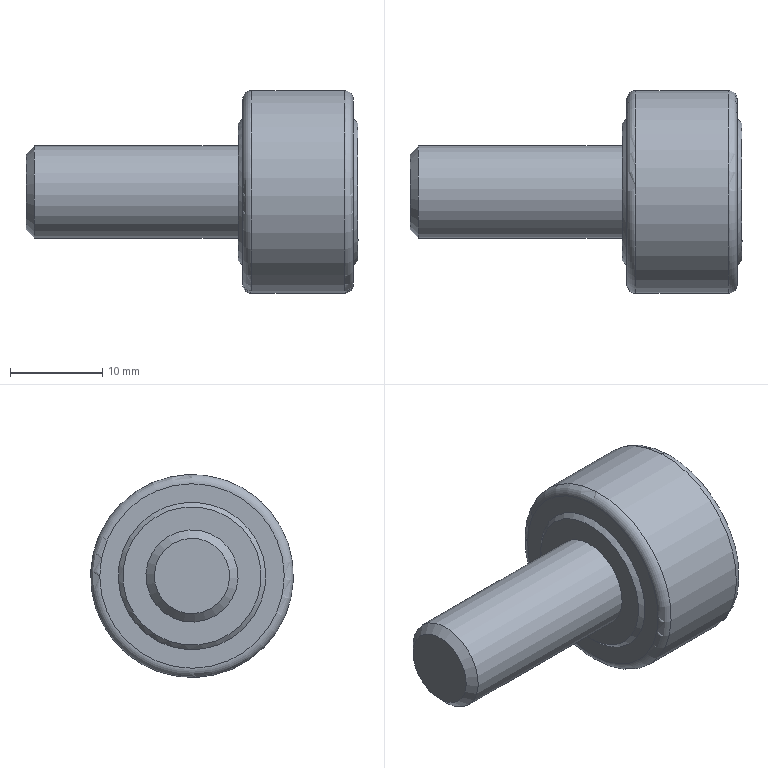Part | NX | features CFFRC10-22 2 | 1 solid | 24 faces | box 36 x 22 x 22 mm | volume 6364 mm3 | plane 14 | cone 4 | cylinder 4 | torus 2 | commonest cylinder face diameters 2 x1 4 x1 10 x1 22 x1
STEP:
#1=CARTESIAN_POINT('',(-25.5,-117.523,-671.264));
#2=VERTEX_POINT('',#1);
#3=CARTESIAN_POINT('',(-25.5,-120.421,-674.136));
#4=DIRECTION('',(-1.,0.,0.));
#5=DIRECTION('',(0.,0.7102,0.704));
#6=AXIS2_PLACEMENT_3D('',#3,#4,#5);
#7=CIRCLE('',#6,4.08);
#8=EDGE_CURVE('',#2,#2,#7,.T.);
#9=ORIENTED_EDGE('',*,*,#8,.T.);
#10=EDGE_LOOP('',(#9));
#11=FACE_BOUND('',#10,.T.);
#12=CARTESIAN_POINT('',(-25.5,-121.857,-672.688));
#13=DIRECTION('',(-1.,0.,0.));
#14=DIRECTION('',(0.,-0.7102,-0.704));
#15=AXIS2_PLACEMENT_3D('',#12,#13,#14);
#16=PLANE('',#15);
#17=ADVANCED_FACE('',(#11),#16,.T.);
#18=CARTESIAN_POINT('',(-24.58,-123.972,-677.656));
#19=VERTEX_POINT('',#18);
#20=CARTESIAN_POINT('',(-24.58,-120.421,-674.136));
#21=DIRECTION('',(-1.,0.,0.));
#22=DIRECTION('',(0.,-0.7102,-0.704));
#23=AXIS2_PLACEMENT_3D('',#20,#21,#22);
#24=CIRCLE('',#23,5.);
#25=EDGE_CURVE('',#19,#19,#24,.T.);
#26=ORIENTED_EDGE('',*,*,#25,.T.);
#27=EDGE_LOOP('',(#26));
#28=FACE_BOUND('',#27,.T.);
#29=ORIENTED_EDGE('',*,*,#8,.F.);
#30=EDGE_LOOP('',(#29));
#31=FACE_BOUND('',#30,.T.);
#32=CARTESIAN_POINT('',(-25.54,-120.421,-674.136));
#33=DIRECTION('',(1.,0.,0.));
#34=DIRECTION('',(0.,0.7102,0.704));
#35=AXIS2_PLACEMENT_3D('',#32,#33,#34);
#36=CONICAL_SURFACE('',#35,4.04,0.7854);
#37=ADVANCED_FACE('',(#28,#31),#36,.T.);
#38=ORIENTED_EDGE('',*,*,#25,.F.);
#39=EDGE_LOOP('',(#38));
#40=FACE_BOUND('',#39,.T.);
#41=CARTESIAN_POINT('',(-2.5,-116.87,-670.616));
#42=VERTEX_POINT('',#41);
#43=CARTESIAN_POINT('',(-2.5,-120.421,-674.136));
#44=DIRECTION('',(1.,0.,0.));
#45=DIRECTION('',(0.,0.7102,0.704));
#46=AXIS2_PLACEMENT_3D('',#43,#44,#45);
#47=CIRCLE('',#46,5.);
#48=EDGE_CURVE('',#42,#42,#47,.T.);
#49=ORIENTED_EDGE('',*,*,#48,.F.);
#50=EDGE_LOOP('',(#49));
#51=FACE_BOUND('',#50,.T.);
#52=CARTESIAN_POINT('',(-13.54,-120.421,-674.136));
#53=DIRECTION('',(-1.,0.,0.));
#54=DIRECTION('',(0.,-0.7102,-0.704));
#55=AXIS2_PLACEMENT_3D('',#52,#53,#54);
#56=CYLINDRICAL_SURFACE('',#55,5.);
#57=ADVANCED_FACE('',(#40,#51),#56,.T.);
#58=ORIENTED_EDGE('',*,*,#48,.T.);
#59=EDGE_LOOP('',(#58));
#60=FACE_BOUND('',#59,.T.);
#61=CARTESIAN_POINT('',(-2.5,-115.094,-668.856));
#62=VERTEX_POINT('',#61);
#63=CARTESIAN_POINT('',(-2.5,-120.421,-674.136));
#64=DIRECTION('',(-1.,0.,0.));
#65=DIRECTION('',(0.,0.7102,0.704));
#66=AXIS2_PLACEMENT_3D('',#63,#64,#65);
#67=CIRCLE('',#66,7.5);
#68=EDGE_CURVE('',#62,#62,#67,.T.);
#69=ORIENTED_EDGE('',*,*,#68,.T.);
#70=EDGE_LOOP('',(#69));
#71=FACE_BOUND('',#70,.T.);
#72=CARTESIAN_POINT('',(-2.5,-124.821,-669.698));
#73=DIRECTION('',(-1.,0.,0.));
#74=DIRECTION('',(0.,-0.7102,-0.704));
#75=AXIS2_PLACEMENT_3D('',#72,#73,#74);
#76=PLANE('',#75);
#77=ADVANCED_FACE('',(#60,#71),#76,.T.);
#78=ORIENTED_EDGE('',*,*,#68,.F.);
#79=EDGE_LOOP('',(#78));
#80=FACE_BOUND('',#79,.T.);
#81=CARTESIAN_POINT('',(-2.,-126.102,-679.768));
#82=VERTEX_POINT('',#81);
#83=CARTESIAN_POINT('',(-2.,-120.421,-674.136));
#84=DIRECTION('',(1.,0.,0.));
#85=DIRECTION('',(0.,-0.7102,-0.704));
#86=AXIS2_PLACEMENT_3D('',#83,#84,#85);
#87=CIRCLE('',#86,8.);
#88=EDGE_CURVE('',#82,#82,#87,.T.);
#89=ORIENTED_EDGE('',*,*,#88,.F.);
#90=EDGE_LOOP('',(#89));
#91=FACE_BOUND('',#90,.T.);
#92=CARTESIAN_POINT('',(-2.54,-120.421,-674.136));
#93=DIRECTION('',(1.,0.,0.));
#94=DIRECTION('',(0.,0.7102,0.704));
#95=AXIS2_PLACEMENT_3D('',#92,#93,#94);
#96=CONICAL_SURFACE('',#95,7.46,0.7854);
#97=ADVANCED_FACE('',(#80,#91),#96,.T.);
#98=ORIENTED_EDGE('',*,*,#88,.T.);
#99=EDGE_LOOP('',(#98));
#100=FACE_BOUND('',#99,.T.);
#101=CARTESIAN_POINT('',(-2.,-113.319,-667.096));
#102=VERTEX_POINT('',#101);
#103=CARTESIAN_POINT('',(-2.,-120.421,-674.136));
#104=DIRECTION('',(-1.,0.,0.));
#105=DIRECTION('',(0.,0.7102,0.704));
#106=AXIS2_PLACEMENT_3D('',#103,#104,#105);
#107=CIRCLE('',#106,10.);
#108=EDGE_CURVE('',#102,#102,#107,.T.);
#109=ORIENTED_EDGE('',*,*,#108,.T.);
#110=EDGE_LOOP('',(#109));
#111=FACE_BOUND('',#110,.T.);
#112=CARTESIAN_POINT('',(-2.,-126.757,-667.745));
#113=DIRECTION('',(-1.,0.,0.));
#114=DIRECTION('',(0.,-0.704,0.7102));
#115=AXIS2_PLACEMENT_3D('',#112,#113,#114);
#116=PLANE('',#115);
#117=ADVANCED_FACE('',(#100,#111),#116,.T.);
#118=CARTESIAN_POINT('',(4.,-123.935,-669.171));
#119=VERTEX_POINT('',#118);
#120=CARTESIAN_POINT('',(4.,-124.645,-669.875));
#121=DIRECTION('',(0.,0.704,-0.7102));
#122=DIRECTION('',(0.,0.7102,0.704));
#123=AXIS2_PLACEMENT_3D('',#120,#121,#122);
#124=CIRCLE('',#123,1.);
#125=EDGE_CURVE('',#119,#119,#124,.T.);
#126=ORIENTED_EDGE('',*,*,#125,.T.);
#127=EDGE_LOOP('',(#126));
#128=FACE_BOUND('',#127,.T.);
#129=CARTESIAN_POINT('',(4.5,-124.645,-669.875));
#130=DIRECTION('',(0.,-0.704,0.7102));
#131=DIRECTION('',(0.,0.7102,0.704));
#132=AXIS2_PLACEMENT_3D('',#129,#130,#131);
#133=PLANE('',#132);
#134=ADVANCED_FACE('',(#128),#133,.F.);
#135=CARTESIAN_POINT('',(4.,-120.93,-672.202));
#136=VERTEX_POINT('',#135);
#137=CARTESIAN_POINT('',(4.,-122.35,-673.61));
#138=VERTEX_POINT('',#137);
#139=CARTESIAN_POINT('',(4.,-120.93,-672.202));
#140=CARTESIAN_POINT('',(3.465,-120.928,-672.204));
#141=CARTESIAN_POINT('',(2.535,-122.019,-672.524));
#142=CARTESIAN_POINT('',(3.465,-122.349,-673.612));
#143=CARTESIAN_POINT('',(4.,-122.35,-673.61));
#144=B_SPLINE_CURVE_WITH_KNOTS('',3,(#139,#140,#141,#142,#143),.UNSPECIFIED.,.F.,.F.,(4,1,4),(0.,0.5,1.),.UNSPECIFIED.);
#145=EDGE_CURVE('',#136,#138,#144,.T.);
#146=ORIENTED_EDGE('',*,*,#145,.F.);
#147=CARTESIAN_POINT('',(4.,-122.35,-673.61));
#148=CARTESIAN_POINT('',(4.535,-122.349,-673.612));
#149=CARTESIAN_POINT('',(5.465,-122.019,-672.524));
#150=CARTESIAN_POINT('',(4.535,-120.928,-672.204));
#151=CARTESIAN_POINT('',(4.,-120.93,-672.202));
#152=B_SPLINE_CURVE_WITH_KNOTS('',3,(#147,#148,#149,#150,#151),.UNSPECIFIED.,.F.,.F.,(4,1,4),(0.,0.5,1.),.UNSPECIFIED.);
#153=EDGE_CURVE('',#138,#136,#152,.T.);
#154=ORIENTED_EDGE('',*,*,#153,.F.);
#155=EDGE_LOOP('',(#146,#154));
#156=FACE_BOUND('',#155,.T.);
#157=ORIENTED_EDGE('',*,*,#125,.F.);
#158=EDGE_LOOP('',(#157));
#159=FACE_BOUND('',#158,.T.);
#160=CARTESIAN_POINT('',(4.,-122.885,-671.651));
#161=DIRECTION('',(0.,-0.704,0.7102));
#162=DIRECTION('',(0.,0.7102,0.704));
#163=AXIS2_PLACEMENT_3D('',#160,#161,#162);
#164=CYLINDRICAL_SURFACE('',#163,1.);
#165=ADVANCED_FACE('',(#156,#159),#164,.F.);
#166=CARTESIAN_POINT('',(2.555,-119.,-672.728));
#167=VERTEX_POINT('',#166);
#168=CARTESIAN_POINT('',(2.555,-120.421,-674.136));
#169=DIRECTION('',(1.,0.,0.));
#170=DIRECTION('',(0.,0.7102,0.704));
#171=AXIS2_PLACEMENT_3D('',#168,#169,#170);
#172=CIRCLE('',#171,2.);
#173=EDGE_CURVE('',#167,#167,#172,.T.);
#174=ORIENTED_EDGE('',*,*,#173,.T.);
#175=EDGE_LOOP('',(#174));
#176=FACE_BOUND('',#175,.T.);
#177=CARTESIAN_POINT('',(1.4,-120.421,-674.136));
#178=VERTEX_POINT('',#177);
#179=VERTEX_LOOP('',#178);
#180=FACE_BOUND('',#179,.T.);
#181=CARTESIAN_POINT('',(1.4,-120.421,-674.136));
#182=DIRECTION('',(1.,0.,0.));
#183=DIRECTION('',(0.,0.7102,0.704));
#184=AXIS2_PLACEMENT_3D('',#181,#182,#183);
#185=CONICAL_SURFACE('',#184,0.,1.047);
#186=ADVANCED_FACE('',(#176,#180),#185,.F.);
#187=CARTESIAN_POINT('',(10.5,-117.16,-669.613));
#188=VERTEX_POINT('',#187);
#189=CARTESIAN_POINT('',(7.9,-117.16,-669.613));
#190=VERTEX_POINT('',#189);
#191=CARTESIAN_POINT('',(10.5,-117.16,-669.613));
#192=DIRECTION('',(-1.,0.,0.));
#193=VECTOR('',#192,1000.);
#194=LINE('',#191,#193);
#195=EDGE_CURVE('',#188,#190,#194,.T.);
#196=ORIENTED_EDGE('',*,*,#195,.F.);
#197=CARTESIAN_POINT('',(10.5,-119.804,-672.234));
#198=VERTEX_POINT('',#197);
#199=CARTESIAN_POINT('',(10.5,-117.16,-669.613));
#200=DIRECTION('',(0.,-0.7102,-0.704));
#201=VECTOR('',#200,1000.);
#202=LINE('',#199,#201);
#203=EDGE_CURVE('',#188,#198,#202,.T.);
#204=ORIENTED_EDGE('',*,*,#203,.T.);
#205=CARTESIAN_POINT('',(7.9,-119.804,-672.234));
#206=VERTEX_POINT('',#205);
#207=CARTESIAN_POINT('',(7.9,-119.804,-672.234));
#208=DIRECTION('',(1.,0.,0.));
#209=VECTOR('',#208,1000.);
#210=LINE('',#207,#209);
#211=EDGE_CURVE('',#206,#198,#210,.T.);
#212=ORIENTED_EDGE('',*,*,#211,.F.);
#213=CARTESIAN_POINT('',(7.9,-119.804,-672.234));
#214=DIRECTION('',(0.,0.7102,0.704));
#215=VECTOR('',#214,1000.);
#216=LINE('',#213,#215);
#217=EDGE_CURVE('',#206,#190,#216,.T.);
#218=ORIENTED_EDGE('',*,*,#217,.T.);
#219=EDGE_LOOP('',(#196,#204,#212,#218));
#220=FACE_BOUND('',#219,.T.);
#221=CARTESIAN_POINT('',(10.5,-117.16,-669.613));
#222=DIRECTION('',(0.,-0.704,0.7102));
#223=DIRECTION('',(0.,0.7102,0.704));
#224=AXIS2_PLACEMENT_3D('',#221,#222,#223);
#225=PLANE('',#224);
#226=ADVANCED_FACE('',(#220),#225,.F.);
#227=CARTESIAN_POINT('',(10.5,-115.869,-670.915));
#228=VERTEX_POINT('',#227);
#229=CARTESIAN_POINT('',(7.9,-115.869,-670.915));
#230=VERTEX_POINT('',#229);
#231=CARTESIAN_POINT('',(10.5,-115.869,-670.915));
#232=DIRECTION('',(-1.,0.,0.));
#233=VECTOR('',#232,1000.);
#234=LINE('',#231,#233);
#235=EDGE_CURVE('',#228,#230,#234,.T.);
#236=ORIENTED_EDGE('',*,*,#235,.T.);
#237=CARTESIAN_POINT('',(7.9,-118.513,-673.536));
#238=VERTEX_POINT('',#237);
#239=CARTESIAN_POINT('',(7.9,-115.869,-670.915));
#240=DIRECTION('',(0.,-0.7102,-0.704));
#241=VECTOR('',#240,1000.);
#242=LINE('',#239,#241);
#243=EDGE_CURVE('',#230,#238,#242,.T.);
#244=ORIENTED_EDGE('',*,*,#243,.T.);
#245=CARTESIAN_POINT('',(10.5,-118.513,-673.536));
#246=VERTEX_POINT('',#245);
#247=CARTESIAN_POINT('',(10.5,-118.513,-673.536));
#248=DIRECTION('',(-1.,0.,0.));
#249=VECTOR('',#248,1000.);
#250=LINE('',#247,#249);
#251=EDGE_CURVE('',#246,#238,#250,.T.);
#252=ORIENTED_EDGE('',*,*,#251,.F.);
#253=CARTESIAN_POINT('',(10.5,-118.513,-673.536));
#254=DIRECTION('',(0.,0.7102,0.704));
#255=VECTOR('',#254,1000.);
#256=LINE('',#253,#255);
#257=EDGE_CURVE('',#246,#228,#256,.T.);
#258=ORIENTED_EDGE('',*,*,#257,.T.);
#259=EDGE_LOOP('',(#236,#244,#252,#258));
#260=FACE_BOUND('',#259,.T.);
#261=CARTESIAN_POINT('',(10.5,-123.681,-678.659));
#262=DIRECTION('',(0.,0.704,-0.7102));
#263=DIRECTION('',(0.,-0.7102,-0.704));
#264=AXIS2_PLACEMENT_3D('',#261,#262,#263);
#265=PLANE('',#264);
#266=ADVANCED_FACE('',(#260),#265,.F.);
#267=CARTESIAN_POINT('',(10.5,-115.869,-670.915));
#268=DIRECTION('',(0.,-0.704,0.7102));
#269=VECTOR('',#268,1000.);
#270=LINE('',#267,#269);
#271=EDGE_CURVE('',#228,#188,#270,.T.);
#272=ORIENTED_EDGE('',*,*,#271,.T.);
#273=ORIENTED_EDGE('',*,*,#195,.T.);
#274=CARTESIAN_POINT('',(7.9,-117.16,-669.613));
#275=DIRECTION('',(0.,0.704,-0.7102));
#276=VECTOR('',#275,1000.);
#277=LINE('',#274,#276);
#278=EDGE_CURVE('',#190,#230,#277,.T.);
#279=ORIENTED_EDGE('',*,*,#278,.T.);
#280=ORIENTED_EDGE('',*,*,#235,.F.);
#281=EDGE_LOOP('',(#272,#273,#279,#280));
#282=FACE_BOUND('',#281,.T.);
#283=CARTESIAN_POINT('',(10.5,-115.869,-670.915));
#284=DIRECTION('',(0.,0.7102,0.704));
#285=DIRECTION('',(-1.,0.,0.));
#286=AXIS2_PLACEMENT_3D('',#283,#284,#285);
#287=PLANE('',#286);
#288=ADVANCED_FACE('',(#282),#287,.F.);
#289=ORIENTED_EDGE('',*,*,#217,.F.);
#290=CARTESIAN_POINT('',(7.9,-120.421,-674.136));
#291=DIRECTION('',(-1.,0.,0.));
#292=DIRECTION('',(0.,0.3085,0.9512));
#293=AXIS2_PLACEMENT_3D('',#290,#291,#292);
#294=CIRCLE('',#293,2.);
#295=EDGE_CURVE('',#206,#238,#294,.T.);
#296=ORIENTED_EDGE('',*,*,#295,.T.);
#297=ORIENTED_EDGE('',*,*,#243,.F.);
#298=ORIENTED_EDGE('',*,*,#278,.F.);
#299=EDGE_LOOP('',(#289,#296,#297,#298));
#300=FACE_BOUND('',#299,.T.);
#301=CARTESIAN_POINT('',(7.9,-120.421,-674.136));
#302=DIRECTION('',(1.,0.,0.));
#303=DIRECTION('',(0.,0.7102,0.704));
#304=AXIS2_PLACEMENT_3D('',#301,#302,#303);
#305=PLANE('',#304);
#306=ADVANCED_FACE('',(#300),#305,.T.);
#307=ORIENTED_EDGE('',*,*,#173,.F.);
#308=EDGE_LOOP('',(#307));
#309=FACE_BOUND('',#308,.T.);
#310=ORIENTED_EDGE('',*,*,#145,.T.);
#311=ORIENTED_EDGE('',*,*,#153,.T.);
#312=EDGE_LOOP('',(#310,#311));
#313=FACE_BOUND('',#312,.T.);
#314=ORIENTED_EDGE('',*,*,#295,.F.);
#315=ORIENTED_EDGE('',*,*,#211,.T.);
#316=CARTESIAN_POINT('',(10.5,-122.328,-674.737));
#317=VERTEX_POINT('',#316);
#318=CARTESIAN_POINT('',(10.5,-120.421,-674.136));
#319=DIRECTION('',(-1.,0.,0.));
#320=DIRECTION('',(0.,-0.9539,-0.3002));
#321=AXIS2_PLACEMENT_3D('',#318,#319,#320);
#322=CIRCLE('',#321,2.);
#323=EDGE_CURVE('',#317,#198,#322,.T.);
#324=ORIENTED_EDGE('',*,*,#323,.F.);
#325=CARTESIAN_POINT('',(7.9,-122.328,-674.737));
#326=VERTEX_POINT('',#325);
#327=CARTESIAN_POINT('',(10.5,-122.328,-674.737));
#328=DIRECTION('',(-1.,0.,0.));
#329=VECTOR('',#328,1000.);
#330=LINE('',#327,#329);
#331=EDGE_CURVE('',#317,#326,#330,.T.);
#332=ORIENTED_EDGE('',*,*,#331,.T.);
#333=CARTESIAN_POINT('',(7.9,-121.038,-676.039));
#334=VERTEX_POINT('',#333);
#335=CARTESIAN_POINT('',(7.9,-120.421,-674.136));
#336=DIRECTION('',(-1.,0.,0.));
#337=DIRECTION('',(0.,-0.7102,-0.704));
#338=AXIS2_PLACEMENT_3D('',#335,#336,#337);
#339=CIRCLE('',#338,2.);
#340=EDGE_CURVE('',#334,#326,#339,.T.);
#341=ORIENTED_EDGE('',*,*,#340,.F.);
#342=CARTESIAN_POINT('',(10.5,-121.038,-676.039));
#343=VERTEX_POINT('',#342);
#344=CARTESIAN_POINT('',(7.9,-121.038,-676.039));
#345=DIRECTION('',(1.,0.,0.));
#346=VECTOR('',#345,1000.);
#347=LINE('',#344,#346);
#348=EDGE_CURVE('',#334,#343,#347,.T.);
#349=ORIENTED_EDGE('',*,*,#348,.T.);
#350=CARTESIAN_POINT('',(10.5,-120.421,-674.136));
#351=DIRECTION('',(-1.,0.,0.));
#352=DIRECTION('',(0.,0.9539,0.3002));
#353=AXIS2_PLACEMENT_3D('',#350,#351,#352);
#354=CIRCLE('',#353,2.);
#355=EDGE_CURVE('',#246,#343,#354,.T.);
#356=ORIENTED_EDGE('',*,*,#355,.F.);
#357=ORIENTED_EDGE('',*,*,#251,.T.);
#358=EDGE_LOOP('',(#314,#315,#324,#332,#341,#349,#356,#357));
#359=FACE_BOUND('',#358,.T.);
#360=CARTESIAN_POINT('',(6.527,-120.421,-674.136));
#361=DIRECTION('',(-1.,0.,0.));
#362=DIRECTION('',(0.,-0.7102,-0.704));
#363=AXIS2_PLACEMENT_3D('',#360,#361,#362);
#364=CYLINDRICAL_SURFACE('',#363,2.);
#365=ADVANCED_FACE('',(#309,#313,#359),#364,.F.);
#366=CARTESIAN_POINT('',(7.9,-124.972,-677.357));
#367=VERTEX_POINT('',#366);
#368=CARTESIAN_POINT('',(10.5,-124.972,-677.357));
#369=VERTEX_POINT('',#368);
#370=CARTESIAN_POINT('',(7.9,-124.972,-677.357));
#371=DIRECTION('',(1.,0.,0.));
#372=VECTOR('',#371,1000.);
#373=LINE('',#370,#372);
#374=EDGE_CURVE('',#367,#369,#373,.T.);
#375=ORIENTED_EDGE('',*,*,#374,.F.);
#376=CARTESIAN_POINT('',(7.9,-124.972,-677.357));
#377=DIRECTION('',(0.,0.7102,0.704));
#378=VECTOR('',#377,1000.);
#379=LINE('',#376,#378);
#380=EDGE_CURVE('',#367,#326,#379,.T.);
#381=ORIENTED_EDGE('',*,*,#380,.T.);
#382=ORIENTED_EDGE('',*,*,#331,.F.);
#383=CARTESIAN_POINT('',(10.5,-122.328,-674.737));
#384=DIRECTION('',(0.,-0.7102,-0.704));
#385=VECTOR('',#384,1000.);
#386=LINE('',#383,#385);
#387=EDGE_CURVE('',#317,#369,#386,.T.);
#388=ORIENTED_EDGE('',*,*,#387,.T.);
#389=EDGE_LOOP('',(#375,#381,#382,#388));
#390=FACE_BOUND('',#389,.T.);
#391=CARTESIAN_POINT('',(10.5,-117.16,-669.613));
#392=DIRECTION('',(0.,-0.704,0.7102));
#393=DIRECTION('',(0.,0.7102,0.704));
#394=AXIS2_PLACEMENT_3D('',#391,#392,#393);
#395=PLANE('',#394);
#396=ADVANCED_FACE('',(#390),#395,.F.);
#397=CARTESIAN_POINT('',(10.5,-123.681,-678.659));
#398=VERTEX_POINT('',#397);
#399=CARTESIAN_POINT('',(10.5,-124.972,-677.357));
#400=DIRECTION('',(0.,0.704,-0.7102));
#401=VECTOR('',#400,1000.);
#402=LINE('',#399,#401);
#403=EDGE_CURVE('',#369,#398,#402,.T.);
#404=ORIENTED_EDGE('',*,*,#403,.T.);
#405=CARTESIAN_POINT('',(7.9,-123.681,-678.659));
#406=VERTEX_POINT('',#405);
#407=CARTESIAN_POINT('',(10.5,-123.681,-678.659));
#408=DIRECTION('',(-1.,0.,0.));
#409=VECTOR('',#408,1000.);
#410=LINE('',#407,#409);
#411=EDGE_CURVE('',#398,#406,#410,.T.);
#412=ORIENTED_EDGE('',*,*,#411,.T.);
#413=CARTESIAN_POINT('',(7.9,-123.681,-678.659));
#414=DIRECTION('',(0.,-0.704,0.7102));
#415=VECTOR('',#414,1000.);
#416=LINE('',#413,#415);
#417=EDGE_CURVE('',#406,#367,#416,.T.);
#418=ORIENTED_EDGE('',*,*,#417,.T.);
#419=ORIENTED_EDGE('',*,*,#374,.T.);
#420=EDGE_LOOP('',(#404,#412,#418,#419));
#421=FACE_BOUND('',#420,.T.);
#422=CARTESIAN_POINT('',(10.5,-124.972,-677.357));
#423=DIRECTION('',(0.,-0.7102,-0.704));
#424=DIRECTION('',(1.,0.,0.));
#425=AXIS2_PLACEMENT_3D('',#422,#423,#424);
#426=PLANE('',#425);
#427=ADVANCED_FACE('',(#421),#426,.F.);
#428=CARTESIAN_POINT('',(7.9,-121.038,-676.039));
#429=DIRECTION('',(0.,-0.7102,-0.704));
#430=VECTOR('',#429,1000.);
#431=LINE('',#428,#430);
#432=EDGE_CURVE('',#334,#406,#431,.T.);
#433=ORIENTED_EDGE('',*,*,#432,.F.);
#434=ORIENTED_EDGE('',*,*,#340,.T.);
#435=ORIENTED_EDGE('',*,*,#380,.F.);
#436=ORIENTED_EDGE('',*,*,#417,.F.);
#437=EDGE_LOOP('',(#433,#434,#435,#436));
#438=FACE_BOUND('',#437,.T.);
#439=CARTESIAN_POINT('',(7.9,-120.421,-674.136));
#440=DIRECTION('',(1.,0.,0.));
#441=DIRECTION('',(0.,0.7102,0.704));
#442=AXIS2_PLACEMENT_3D('',#439,#440,#441);
#443=PLANE('',#442);
#444=ADVANCED_FACE('',(#438),#443,.T.);
#445=ORIENTED_EDGE('',*,*,#411,.F.);
#446=CARTESIAN_POINT('',(10.5,-123.681,-678.659));
#447=DIRECTION('',(0.,0.7102,0.704));
#448=VECTOR('',#447,1000.);
#449=LINE('',#446,#448);
#450=EDGE_CURVE('',#398,#343,#449,.T.);
#451=ORIENTED_EDGE('',*,*,#450,.T.);
#452=ORIENTED_EDGE('',*,*,#348,.F.);
#453=ORIENTED_EDGE('',*,*,#432,.T.);
#454=EDGE_LOOP('',(#445,#451,#452,#453));
#455=FACE_BOUND('',#454,.T.);
#456=CARTESIAN_POINT('',(10.5,-123.681,-678.659));
#457=DIRECTION('',(0.,0.704,-0.7102));
#458=DIRECTION('',(0.,-0.7102,-0.704));
#459=AXIS2_PLACEMENT_3D('',#456,#457,#458);
#460=PLANE('',#459);
#461=ADVANCED_FACE('',(#455),#460,.F.);
#462=ORIENTED_EDGE('',*,*,#403,.F.);
#463=ORIENTED_EDGE('',*,*,#387,.F.);
#464=ORIENTED_EDGE('',*,*,#323,.T.);
#465=ORIENTED_EDGE('',*,*,#203,.F.);
#466=ORIENTED_EDGE('',*,*,#271,.F.);
#467=ORIENTED_EDGE('',*,*,#257,.F.);
#468=ORIENTED_EDGE('',*,*,#355,.T.);
#469=ORIENTED_EDGE('',*,*,#450,.F.);
#470=EDGE_LOOP('',(#462,#463,#464,#465,#466,#467,#468,#469));
#471=FACE_BOUND('',#470,.T.);
#472=CARTESIAN_POINT('',(10.5,-115.094,-668.856));
#473=VERTEX_POINT('',#472);
#474=CARTESIAN_POINT('',(10.5,-120.421,-674.136));
#475=DIRECTION('',(1.,0.,0.));
#476=DIRECTION('',(0.,0.7102,0.704));
#477=AXIS2_PLACEMENT_3D('',#474,#475,#476);
#478=CIRCLE('',#477,7.5);
#479=EDGE_CURVE('',#473,#473,#478,.T.);
#480=ORIENTED_EDGE('',*,*,#479,.T.);
#481=EDGE_LOOP('',(#480));
#482=FACE_BOUND('',#481,.T.);
#483=CARTESIAN_POINT('',(10.5,-123.061,-671.473));
#484=DIRECTION('',(1.,0.,0.));
#485=DIRECTION('',(0.,0.7102,0.704));
#486=AXIS2_PLACEMENT_3D('',#483,#484,#485);
#487=PLANE('',#486);
#488=ADVANCED_FACE('',(#471,#482),#487,.T.);
#489=ORIENTED_EDGE('',*,*,#479,.F.);
#490=EDGE_LOOP('',(#489));
#491=FACE_BOUND('',#490,.T.);
#492=CARTESIAN_POINT('',(10.,-126.102,-679.768));
#493=VERTEX_POINT('',#492);
#494=CARTESIAN_POINT('',(10.,-120.421,-674.136));
#495=DIRECTION('',(-1.,0.,0.));
#496=DIRECTION('',(0.,-0.7102,-0.704));
#497=AXIS2_PLACEMENT_3D('',#494,#495,#496);
#498=CIRCLE('',#497,8.);
#499=EDGE_CURVE('',#493,#493,#498,.T.);
#500=ORIENTED_EDGE('',*,*,#499,.F.);
#501=EDGE_LOOP('',(#500));
#502=FACE_BOUND('',#501,.T.);
#503=CARTESIAN_POINT('',(10.54,-120.421,-674.136));
#504=DIRECTION('',(-1.,0.,0.));
#505=DIRECTION('',(0.,-0.7102,-0.704));
#506=AXIS2_PLACEMENT_3D('',#503,#504,#505);
#507=CONICAL_SURFACE('',#506,7.46,0.7854);
#508=ADVANCED_FACE('',(#491,#502),#507,.T.);
#509=ORIENTED_EDGE('',*,*,#499,.T.);
#510=EDGE_LOOP('',(#509));
#511=FACE_BOUND('',#510,.T.);
#512=CARTESIAN_POINT('',(10.,-113.319,-667.096));
#513=VERTEX_POINT('',#512);
#514=CARTESIAN_POINT('',(10.,-120.421,-674.136));
#515=DIRECTION('',(1.,0.,0.));
#516=DIRECTION('',(0.,0.7102,0.704));
#517=AXIS2_PLACEMENT_3D('',#514,#515,#516);
#518=CIRCLE('',#517,10.);
#519=EDGE_CURVE('',#513,#513,#518,.T.);
#520=ORIENTED_EDGE('',*,*,#519,.T.);
#521=EDGE_LOOP('',(#520));
#522=FACE_BOUND('',#521,.T.);
#523=CARTESIAN_POINT('',(10.,-126.757,-667.745));
#524=DIRECTION('',(1.,0.,0.));
#525=DIRECTION('',(0.,0.7102,0.704));
#526=AXIS2_PLACEMENT_3D('',#523,#524,#525);
#527=PLANE('',#526);
#528=ADVANCED_FACE('',(#511,#522),#527,.T.);
#529=ORIENTED_EDGE('',*,*,#519,.F.);
#530=EDGE_LOOP('',(#529));
#531=FACE_BOUND('',#530,.T.);
#532=CARTESIAN_POINT('',(9.,-128.233,-681.88));
#533=VERTEX_POINT('',#532);
#534=CARTESIAN_POINT('',(9.,-120.421,-674.136));
#535=DIRECTION('',(1.,0.,0.));
#536=DIRECTION('',(0.,-0.7102,-0.704));
#537=AXIS2_PLACEMENT_3D('',#534,#535,#536);
#538=CIRCLE('',#537,11.);
#539=EDGE_CURVE('',#533,#533,#538,.T.);
#540=ORIENTED_EDGE('',*,*,#539,.T.);
#541=EDGE_LOOP('',(#540));
#542=FACE_BOUND('',#541,.T.);
#543=CARTESIAN_POINT('',(9.,-120.421,-674.136));
#544=DIRECTION('',(-1.,0.,0.));
#545=DIRECTION('',(0.,0.7102,0.704));
#546=AXIS2_PLACEMENT_3D('',#543,#544,#545);
#547=TOROIDAL_SURFACE('',#546,10.,1.);
#548=ADVANCED_FACE('',(#531,#542),#547,.T.);
#549=CARTESIAN_POINT('',(-1.,-112.609,-666.392));
#550=VERTEX_POINT('',#549);
#551=CARTESIAN_POINT('',(-1.,-120.421,-674.136));
#552=DIRECTION('',(-1.,0.,0.));
#553=DIRECTION('',(0.,0.7102,0.704));
#554=AXIS2_PLACEMENT_3D('',#551,#552,#553);
#555=CIRCLE('',#554,11.);
#556=EDGE_CURVE('',#550,#550,#555,.T.);
#557=ORIENTED_EDGE('',*,*,#556,.F.);
#558=EDGE_LOOP('',(#557));
#559=FACE_BOUND('',#558,.T.);
#560=ORIENTED_EDGE('',*,*,#539,.F.);
#561=EDGE_LOOP('',(#560));
#562=FACE_BOUND('',#561,.T.);
#563=CARTESIAN_POINT('',(4.,-120.421,-674.136));
#564=DIRECTION('',(-1.,0.,0.));
#565=DIRECTION('',(0.,-0.7102,-0.704));
#566=AXIS2_PLACEMENT_3D('',#563,#564,#565);
#567=CYLINDRICAL_SURFACE('',#566,11.);
#568=ADVANCED_FACE('',(#559,#562),#567,.T.);
#569=ORIENTED_EDGE('',*,*,#108,.F.);
#570=EDGE_LOOP('',(#569));
#571=FACE_BOUND('',#570,.T.);
#572=ORIENTED_EDGE('',*,*,#556,.T.);
#573=EDGE_LOOP('',(#572));
#574=FACE_BOUND('',#573,.T.);
#575=CARTESIAN_POINT('',(-1.,-120.421,-674.136));
#576=DIRECTION('',(-1.,0.,0.));
#577=DIRECTION('',(0.,-0.7102,-0.704));
#578=AXIS2_PLACEMENT_3D('',#575,#576,#577);
#579=TOROIDAL_SURFACE('',#578,10.,1.);
#580=ADVANCED_FACE('',(#571,#574),#579,.T.);
#581=CLOSED_SHELL('',(#17,#37,#57,#77,#97,#117,#134,#165,#186,#226,#266,#288,#306,#365,#396,#427,#444,#461,#488,#508,#528,#548,#568,#580));
#582=MANIFOLD_SOLID_BREP('',#581);
#583=(LENGTH_UNIT()NAMED_UNIT(*)SI_UNIT(.MILLI.,.METRE.));
#584=UNCERTAINTY_MEASURE_WITH_UNIT(LENGTH_MEASURE(0.0508),#583,'','');
#585=(NAMED_UNIT(*)PLANE_ANGLE_UNIT()SI_UNIT($,.RADIAN.));
#586=(NAMED_UNIT(*)SI_UNIT($,.STERADIAN.)SOLID_ANGLE_UNIT());
#587=(GEOMETRIC_REPRESENTATION_CONTEXT(3)GLOBAL_UNCERTAINTY_ASSIGNED_CONTEXT((#584))GLOBAL_UNIT_ASSIGNED_CONTEXT((#583,#585,#586))REPRESENTATION_CONTEXT('',''));
#588=ADVANCED_BREP_SHAPE_REPRESENTATION('',(#582),#587);